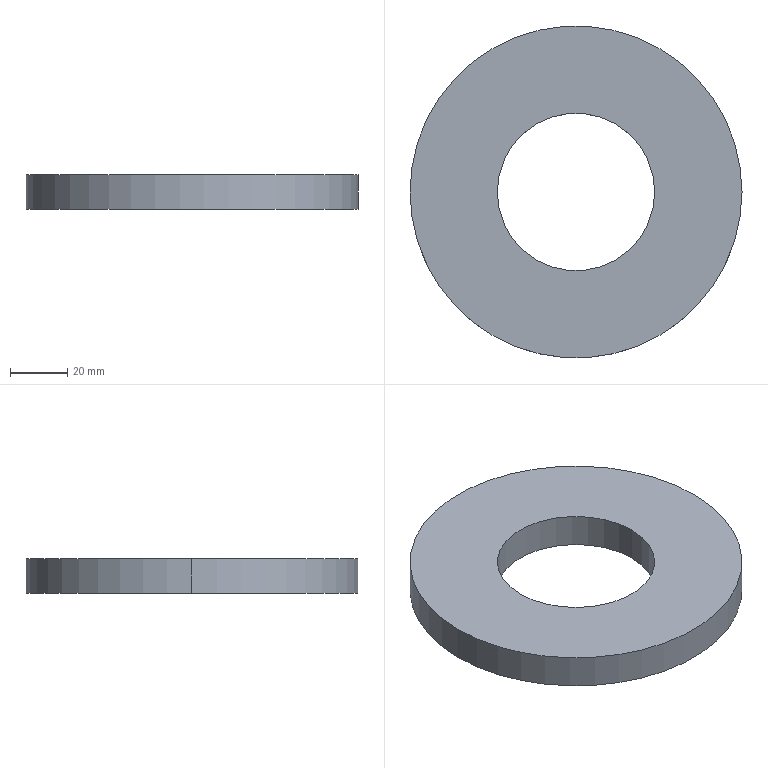Part | SolidWorks | features FlatPattern 1, SMBaseFlange 1, SheetMetal 1 | 1 solid | 6 faces | box 116 x 116 x 12 mm | volume 98310 mm3 | cylinder 4 | plane 2 | commonest cylinder face diameters 55 x2 116 x2
STEP:
#1=CARTESIAN_POINT('',(-27.5,0.,-12.));
#2=VERTEX_POINT('',#1);
#3=CARTESIAN_POINT('',(27.5,0.,-12.));
#4=VERTEX_POINT('',#3);
#5=CARTESIAN_POINT('',(0.,0.,-12.));
#6=DIRECTION('',(0.,0.,1.));
#7=DIRECTION('',(1.,0.,0.));
#8=AXIS2_PLACEMENT_3D('',#5,#6,#7);
#9=CIRCLE('',#8,27.5);
#10=EDGE_CURVE('',#2,#4,#9,.T.);
#11=ORIENTED_EDGE('',*,*,#10,.F.);
#12=CARTESIAN_POINT('',(-27.5,0.,0.));
#13=VERTEX_POINT('',#12);
#14=CARTESIAN_POINT('',(-27.5,0.,-12.));
#15=DIRECTION('',(0.,0.,1.));
#16=VECTOR('',#15,1000.);
#17=LINE('',#14,#16);
#18=EDGE_CURVE('',#2,#13,#17,.T.);
#19=ORIENTED_EDGE('',*,*,#18,.T.);
#20=CARTESIAN_POINT('',(27.5,0.,0.));
#21=VERTEX_POINT('',#20);
#22=CARTESIAN_POINT('',(0.,0.,0.));
#23=DIRECTION('',(0.,0.,1.));
#24=DIRECTION('',(1.,0.,0.));
#25=AXIS2_PLACEMENT_3D('',#22,#23,#24);
#26=CIRCLE('',#25,27.5);
#27=EDGE_CURVE('',#13,#21,#26,.T.);
#28=ORIENTED_EDGE('',*,*,#27,.T.);
#29=CARTESIAN_POINT('',(27.5,0.,-12.));
#30=DIRECTION('',(0.,0.,1.));
#31=VECTOR('',#30,1000.);
#32=LINE('',#29,#31);
#33=EDGE_CURVE('',#4,#21,#32,.T.);
#34=ORIENTED_EDGE('',*,*,#33,.F.);
#35=EDGE_LOOP('',(#11,#19,#28,#34));
#36=FACE_OUTER_BOUND('',#35,.T.);
#37=CARTESIAN_POINT('',(0.,0.,-12.));
#38=DIRECTION('',(0.,0.,1.));
#39=DIRECTION('',(1.,0.,0.));
#40=AXIS2_PLACEMENT_3D('',#37,#38,#39);
#41=CYLINDRICAL_SURFACE('',#40,27.5);
#42=ADVANCED_FACE('',(#36),#41,.F.);
#43=CARTESIAN_POINT('',(58.,0.,-12.));
#44=VERTEX_POINT('',#43);
#45=CARTESIAN_POINT('',(-58.,0.,-12.));
#46=VERTEX_POINT('',#45);
#47=CARTESIAN_POINT('',(0.,0.,-12.));
#48=DIRECTION('',(0.,0.,1.));
#49=DIRECTION('',(1.,0.,0.));
#50=AXIS2_PLACEMENT_3D('',#47,#48,#49);
#51=CIRCLE('',#50,58.);
#52=EDGE_CURVE('',#44,#46,#51,.T.);
#53=ORIENTED_EDGE('',*,*,#52,.T.);
#54=CARTESIAN_POINT('',(-58.,0.,0.));
#55=VERTEX_POINT('',#54);
#56=CARTESIAN_POINT('',(-58.,0.,-12.));
#57=DIRECTION('',(0.,0.,1.));
#58=VECTOR('',#57,1000.);
#59=LINE('',#56,#58);
#60=EDGE_CURVE('',#46,#55,#59,.T.);
#61=ORIENTED_EDGE('',*,*,#60,.T.);
#62=CARTESIAN_POINT('',(58.,0.,0.));
#63=VERTEX_POINT('',#62);
#64=CARTESIAN_POINT('',(0.,0.,0.));
#65=DIRECTION('',(0.,0.,1.));
#66=DIRECTION('',(1.,0.,0.));
#67=AXIS2_PLACEMENT_3D('',#64,#65,#66);
#68=CIRCLE('',#67,58.);
#69=EDGE_CURVE('',#63,#55,#68,.T.);
#70=ORIENTED_EDGE('',*,*,#69,.F.);
#71=CARTESIAN_POINT('',(58.,0.,-12.));
#72=DIRECTION('',(0.,0.,1.));
#73=VECTOR('',#72,1000.);
#74=LINE('',#71,#73);
#75=EDGE_CURVE('',#44,#63,#74,.T.);
#76=ORIENTED_EDGE('',*,*,#75,.F.);
#77=EDGE_LOOP('',(#53,#61,#70,#76));
#78=FACE_OUTER_BOUND('',#77,.T.);
#79=CARTESIAN_POINT('',(0.,0.,-12.));
#80=DIRECTION('',(0.,0.,1.));
#81=DIRECTION('',(1.,0.,0.));
#82=AXIS2_PLACEMENT_3D('',#79,#80,#81);
#83=CYLINDRICAL_SURFACE('',#82,58.);
#84=ADVANCED_FACE('',(#78),#83,.T.);
#85=ORIENTED_EDGE('',*,*,#60,.F.);
#86=CARTESIAN_POINT('',(0.,0.,-12.));
#87=DIRECTION('',(0.,0.,1.));
#88=DIRECTION('',(1.,0.,0.));
#89=AXIS2_PLACEMENT_3D('',#86,#87,#88);
#90=CIRCLE('',#89,58.);
#91=EDGE_CURVE('',#46,#44,#90,.T.);
#92=ORIENTED_EDGE('',*,*,#91,.T.);
#93=ORIENTED_EDGE('',*,*,#75,.T.);
#94=CARTESIAN_POINT('',(0.,0.,0.));
#95=DIRECTION('',(0.,0.,1.));
#96=DIRECTION('',(1.,0.,0.));
#97=AXIS2_PLACEMENT_3D('',#94,#95,#96);
#98=CIRCLE('',#97,58.);
#99=EDGE_CURVE('',#55,#63,#98,.T.);
#100=ORIENTED_EDGE('',*,*,#99,.F.);
#101=EDGE_LOOP('',(#85,#92,#93,#100));
#102=FACE_OUTER_BOUND('',#101,.T.);
#103=CARTESIAN_POINT('',(0.,0.,-12.));
#104=DIRECTION('',(0.,0.,1.));
#105=DIRECTION('',(1.,0.,0.));
#106=AXIS2_PLACEMENT_3D('',#103,#104,#105);
#107=CYLINDRICAL_SURFACE('',#106,58.);
#108=ADVANCED_FACE('',(#102),#107,.T.);
#109=CARTESIAN_POINT('',(0.,0.,-12.));
#110=DIRECTION('',(0.,0.,1.));
#111=DIRECTION('',(1.,0.,0.));
#112=AXIS2_PLACEMENT_3D('',#109,#110,#111);
#113=CIRCLE('',#112,27.5);
#114=EDGE_CURVE('',#4,#2,#113,.T.);
#115=ORIENTED_EDGE('',*,*,#114,.T.);
#116=ORIENTED_EDGE('',*,*,#10,.T.);
#117=EDGE_LOOP('',(#115,#116));
#118=FACE_BOUND('',#117,.T.);
#119=ORIENTED_EDGE('',*,*,#52,.F.);
#120=ORIENTED_EDGE('',*,*,#91,.F.);
#121=EDGE_LOOP('',(#119,#120));
#122=FACE_OUTER_BOUND('',#121,.T.);
#123=CARTESIAN_POINT('',(0.,0.,-12.));
#124=DIRECTION('',(0.,0.,1.));
#125=DIRECTION('',(1.,0.,0.));
#126=AXIS2_PLACEMENT_3D('',#123,#124,#125);
#127=PLANE('',#126);
#128=ADVANCED_FACE('',(#118,#122),#127,.F.);
#129=CARTESIAN_POINT('',(0.,0.,0.));
#130=DIRECTION('',(0.,0.,1.));
#131=DIRECTION('',(1.,0.,0.));
#132=AXIS2_PLACEMENT_3D('',#129,#130,#131);
#133=CIRCLE('',#132,27.5);
#134=EDGE_CURVE('',#21,#13,#133,.T.);
#135=ORIENTED_EDGE('',*,*,#134,.F.);
#136=ORIENTED_EDGE('',*,*,#27,.F.);
#137=EDGE_LOOP('',(#135,#136));
#138=FACE_BOUND('',#137,.T.);
#139=ORIENTED_EDGE('',*,*,#69,.T.);
#140=ORIENTED_EDGE('',*,*,#99,.T.);
#141=EDGE_LOOP('',(#139,#140));
#142=FACE_OUTER_BOUND('',#141,.T.);
#143=CARTESIAN_POINT('',(0.,0.,0.));
#144=DIRECTION('',(0.,0.,1.));
#145=DIRECTION('',(1.,0.,0.));
#146=AXIS2_PLACEMENT_3D('',#143,#144,#145);
#147=PLANE('',#146);
#148=ADVANCED_FACE('',(#138,#142),#147,.T.);
#149=ORIENTED_EDGE('',*,*,#18,.F.);
#150=ORIENTED_EDGE('',*,*,#114,.F.);
#151=ORIENTED_EDGE('',*,*,#33,.T.);
#152=ORIENTED_EDGE('',*,*,#134,.T.);
#153=EDGE_LOOP('',(#149,#150,#151,#152));
#154=FACE_OUTER_BOUND('',#153,.T.);
#155=CARTESIAN_POINT('',(0.,0.,-12.));
#156=DIRECTION('',(0.,0.,1.));
#157=DIRECTION('',(1.,0.,0.));
#158=AXIS2_PLACEMENT_3D('',#155,#156,#157);
#159=CYLINDRICAL_SURFACE('',#158,27.5);
#160=ADVANCED_FACE('',(#154),#159,.F.);
#161=CLOSED_SHELL('',(#42,#84,#108,#128,#148,#160));
#162=MANIFOLD_SOLID_BREP('',#161);
#163=CARTESIAN_POINT('',(0.,0.,0.));
#164=DIRECTION('',(0.,0.,1.));
#165=DIRECTION('',(1.,0.,0.));
#166=AXIS2_PLACEMENT_3D('',#163,#164,#165);
#167=(LENGTH_UNIT()NAMED_UNIT(*)SI_UNIT(.MILLI.,.METRE.));
#168=UNCERTAINTY_MEASURE_WITH_UNIT(LENGTH_MEASURE(0.00001),#167,'','');
#169=(NAMED_UNIT(*)PLANE_ANGLE_UNIT()SI_UNIT($,.RADIAN.));
#170=(NAMED_UNIT(*)SI_UNIT($,.STERADIAN.)SOLID_ANGLE_UNIT());
#171=(GEOMETRIC_REPRESENTATION_CONTEXT(3)GLOBAL_UNCERTAINTY_ASSIGNED_CONTEXT((#168))GLOBAL_UNIT_ASSIGNED_CONTEXT((#167,#169,#170))REPRESENTATION_CONTEXT('',''));
#172=ADVANCED_BREP_SHAPE_REPRESENTATION('',(#162,#166),#171);